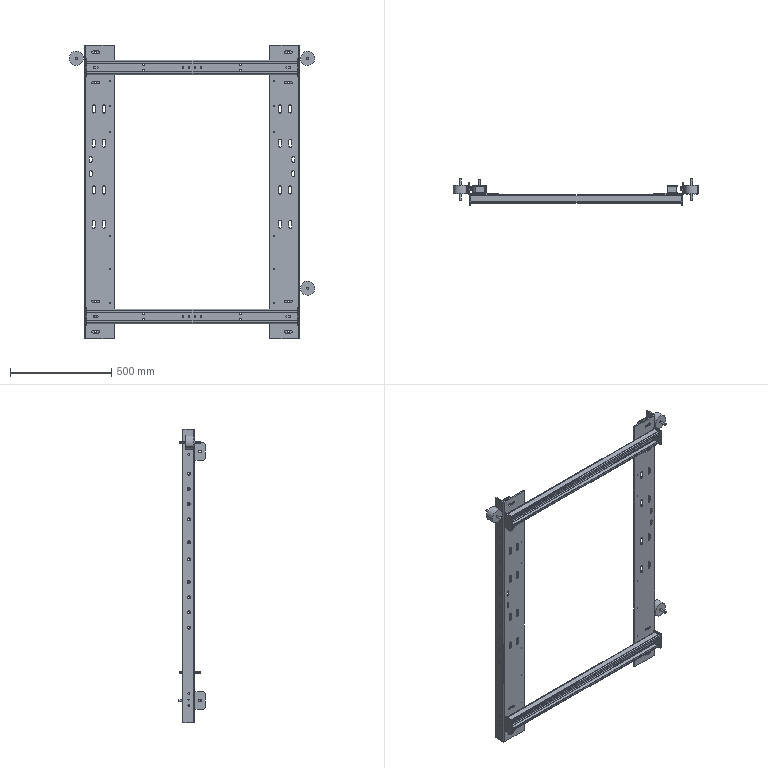Part | SolidWorks | features ReferencePattern 16, LocalLPattern 4, MirrorCompFeat 2 | 36 solids | 1122 faces | box 1212 x 129 x 1450 mm | volume 5699536 mm3 | plane 586 | cylinder 416 | cone 120 | commonest cylinder face diameters 11 x64 14 x48 10.647 x40 14.75 x40 15 x40 15.07 x40